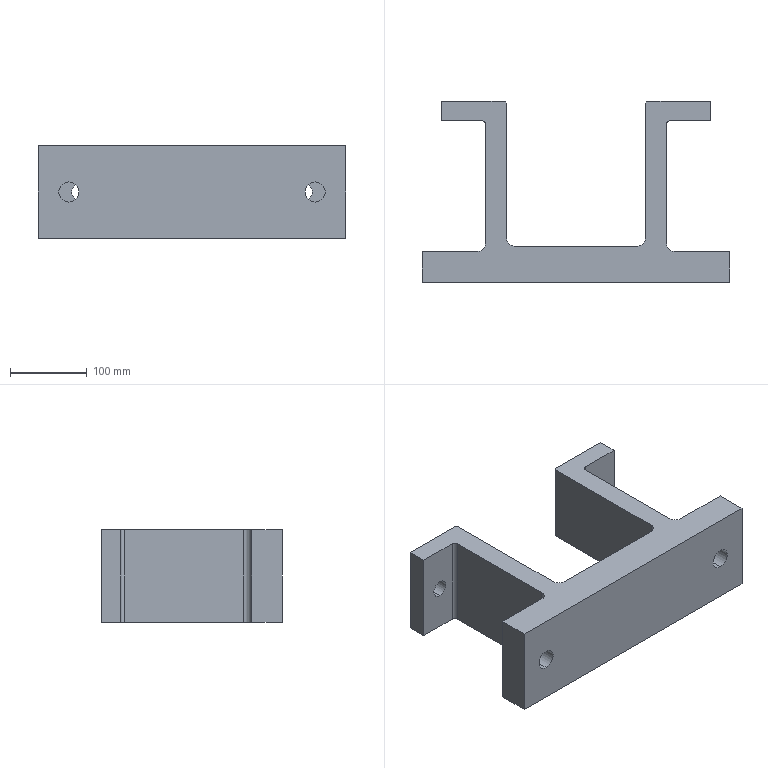Part | SolidWorks | features ICE 3, Extrusion 1 | 1 solid | 42 faces | box 400 x 235 x 120 mm | volume 3581826 mm3 | plane 25 | cylinder 17 | commonest cylinder face diameters 20 x4 22 x4 26 x4 210 x3 10 x2
STEP:
#1=CARTESIAN_POINT('',(145.,210.,-11.));
#2=VERTEX_POINT('',#1);
#3=CARTESIAN_POINT('',(145.,210.,11.));
#4=VERTEX_POINT('',#3);
#5=CARTESIAN_POINT('',(145.,210.,0.));
#6=DIRECTION('',(0.,1.,0.));
#7=DIRECTION('',(-1.,0.,0.));
#8=AXIS2_PLACEMENT_3D('',#5,#6,#7);
#9=CIRCLE('',#8,11.);
#10=EDGE_CURVE('',#2,#4,#9,.T.);
#11=ORIENTED_EDGE('',*,*,#10,.F.);
#12=CARTESIAN_POINT('',(145.,235.,-11.));
#13=VERTEX_POINT('',#12);
#14=CARTESIAN_POINT('',(145.,148.,-11.));
#15=DIRECTION('',(0.,1.,0.));
#16=VECTOR('',#15,1000.);
#17=LINE('',#14,#16);
#18=EDGE_CURVE('',#2,#13,#17,.T.);
#19=ORIENTED_EDGE('',*,*,#18,.T.);
#20=CARTESIAN_POINT('',(145.,235.,11.));
#21=VERTEX_POINT('',#20);
#22=CARTESIAN_POINT('',(145.,235.,0.));
#23=DIRECTION('',(0.,1.,0.));
#24=DIRECTION('',(0.,0.,-1.));
#25=AXIS2_PLACEMENT_3D('',#22,#23,#24);
#26=CIRCLE('',#25,11.);
#27=EDGE_CURVE('',#13,#21,#26,.T.);
#28=ORIENTED_EDGE('',*,*,#27,.T.);
#29=CARTESIAN_POINT('',(145.,148.,11.));
#30=DIRECTION('',(0.,1.,0.));
#31=VECTOR('',#30,1000.);
#32=LINE('',#29,#31);
#33=EDGE_CURVE('',#4,#21,#32,.T.);
#34=ORIENTED_EDGE('',*,*,#33,.F.);
#35=EDGE_LOOP('',(#11,#19,#28,#34));
#36=FACE_OUTER_BOUND('',#35,.T.);
#37=CARTESIAN_POINT('',(145.,148.,0.));
#38=DIRECTION('',(0.,1.,0.));
#39=DIRECTION('',(0.,0.,1.));
#40=AXIS2_PLACEMENT_3D('',#37,#38,#39);
#41=CYLINDRICAL_SURFACE('',#40,11.);
#42=ADVANCED_FACE('',(#36),#41,.F.);
#43=CARTESIAN_POINT('',(-145.,210.,-11.));
#44=VERTEX_POINT('',#43);
#45=CARTESIAN_POINT('',(-145.,210.,11.));
#46=VERTEX_POINT('',#45);
#47=CARTESIAN_POINT('',(-145.,210.,0.));
#48=DIRECTION('',(0.,1.,0.));
#49=DIRECTION('',(-1.,0.,0.));
#50=AXIS2_PLACEMENT_3D('',#47,#48,#49);
#51=CIRCLE('',#50,11.);
#52=EDGE_CURVE('',#44,#46,#51,.T.);
#53=ORIENTED_EDGE('',*,*,#52,.F.);
#54=CARTESIAN_POINT('',(-145.,235.,-11.));
#55=VERTEX_POINT('',#54);
#56=CARTESIAN_POINT('',(-145.,148.,-11.));
#57=DIRECTION('',(0.,1.,0.));
#58=VECTOR('',#57,1000.);
#59=LINE('',#56,#58);
#60=EDGE_CURVE('',#44,#55,#59,.T.);
#61=ORIENTED_EDGE('',*,*,#60,.T.);
#62=CARTESIAN_POINT('',(-145.,235.,11.));
#63=VERTEX_POINT('',#62);
#64=CARTESIAN_POINT('',(-145.,235.,0.));
#65=DIRECTION('',(0.,1.,0.));
#66=DIRECTION('',(0.,0.,1.));
#67=AXIS2_PLACEMENT_3D('',#64,#65,#66);
#68=CIRCLE('',#67,11.);
#69=EDGE_CURVE('',#55,#63,#68,.T.);
#70=ORIENTED_EDGE('',*,*,#69,.T.);
#71=CARTESIAN_POINT('',(-145.,148.,11.));
#72=DIRECTION('',(0.,1.,0.));
#73=VECTOR('',#72,1000.);
#74=LINE('',#71,#73);
#75=EDGE_CURVE('',#46,#63,#74,.T.);
#76=ORIENTED_EDGE('',*,*,#75,.F.);
#77=EDGE_LOOP('',(#53,#61,#70,#76));
#78=FACE_OUTER_BOUND('',#77,.T.);
#79=CARTESIAN_POINT('',(-145.,148.,0.));
#80=DIRECTION('',(0.,1.,0.));
#81=DIRECTION('',(0.,0.,1.));
#82=AXIS2_PLACEMENT_3D('',#79,#80,#81);
#83=CYLINDRICAL_SURFACE('',#82,11.);
#84=ADVANCED_FACE('',(#78),#83,.F.);
#85=CARTESIAN_POINT('',(-160.,40.,13.));
#86=VERTEX_POINT('',#85);
#87=CARTESIAN_POINT('',(-160.,40.,-13.));
#88=VERTEX_POINT('',#87);
#89=CARTESIAN_POINT('',(-160.,40.,0.));
#90=DIRECTION('',(0.,-1.,0.));
#91=DIRECTION('',(0.,0.,-1.));
#92=AXIS2_PLACEMENT_3D('',#89,#90,#91);
#93=CIRCLE('',#92,13.);
#94=EDGE_CURVE('',#86,#88,#93,.T.);
#95=ORIENTED_EDGE('',*,*,#94,.F.);
#96=CARTESIAN_POINT('',(-160.,0.,13.));
#97=VERTEX_POINT('',#96);
#98=CARTESIAN_POINT('',(-160.,87.,13.));
#99=DIRECTION('',(0.,-1.,0.));
#100=VECTOR('',#99,1000.);
#101=LINE('',#98,#100);
#102=EDGE_CURVE('',#86,#97,#101,.T.);
#103=ORIENTED_EDGE('',*,*,#102,.T.);
#104=CARTESIAN_POINT('',(-160.,0.,-13.));
#105=VERTEX_POINT('',#104);
#106=CARTESIAN_POINT('',(-160.,0.,0.));
#107=DIRECTION('',(0.,-1.,0.));
#108=DIRECTION('',(0.,0.,-1.));
#109=AXIS2_PLACEMENT_3D('',#106,#107,#108);
#110=CIRCLE('',#109,13.);
#111=EDGE_CURVE('',#97,#105,#110,.T.);
#112=ORIENTED_EDGE('',*,*,#111,.T.);
#113=CARTESIAN_POINT('',(-160.,87.,-13.));
#114=DIRECTION('',(0.,-1.,0.));
#115=VECTOR('',#114,1000.);
#116=LINE('',#113,#115);
#117=EDGE_CURVE('',#88,#105,#116,.T.);
#118=ORIENTED_EDGE('',*,*,#117,.F.);
#119=EDGE_LOOP('',(#95,#103,#112,#118));
#120=FACE_OUTER_BOUND('',#119,.T.);
#121=CARTESIAN_POINT('',(-160.,87.,0.));
#122=DIRECTION('',(0.,-1.,0.));
#123=DIRECTION('',(0.,0.,-1.));
#124=AXIS2_PLACEMENT_3D('',#121,#122,#123);
#125=CYLINDRICAL_SURFACE('',#124,13.);
#126=ADVANCED_FACE('',(#120),#125,.F.);
#127=CARTESIAN_POINT('',(160.,40.,13.));
#128=VERTEX_POINT('',#127);
#129=CARTESIAN_POINT('',(160.,40.,-13.));
#130=VERTEX_POINT('',#129);
#131=CARTESIAN_POINT('',(160.,40.,0.));
#132=DIRECTION('',(0.,-1.,0.));
#133=DIRECTION('',(0.,0.,-1.));
#134=AXIS2_PLACEMENT_3D('',#131,#132,#133);
#135=CIRCLE('',#134,13.);
#136=EDGE_CURVE('',#128,#130,#135,.T.);
#137=ORIENTED_EDGE('',*,*,#136,.F.);
#138=CARTESIAN_POINT('',(160.,0.,13.));
#139=VERTEX_POINT('',#138);
#140=CARTESIAN_POINT('',(160.,87.,13.));
#141=DIRECTION('',(0.,-1.,0.));
#142=VECTOR('',#141,1000.);
#143=LINE('',#140,#142);
#144=EDGE_CURVE('',#128,#139,#143,.T.);
#145=ORIENTED_EDGE('',*,*,#144,.T.);
#146=CARTESIAN_POINT('',(160.,0.,-13.));
#147=VERTEX_POINT('',#146);
#148=CARTESIAN_POINT('',(160.,0.,0.));
#149=DIRECTION('',(0.,-1.,0.));
#150=DIRECTION('',(0.,0.,1.));
#151=AXIS2_PLACEMENT_3D('',#148,#149,#150);
#152=CIRCLE('',#151,13.);
#153=EDGE_CURVE('',#139,#147,#152,.T.);
#154=ORIENTED_EDGE('',*,*,#153,.T.);
#155=CARTESIAN_POINT('',(160.,87.,-13.));
#156=DIRECTION('',(0.,-1.,0.));
#157=VECTOR('',#156,1000.);
#158=LINE('',#155,#157);
#159=EDGE_CURVE('',#130,#147,#158,.T.);
#160=ORIENTED_EDGE('',*,*,#159,.F.);
#161=EDGE_LOOP('',(#137,#145,#154,#160));
#162=FACE_OUTER_BOUND('',#161,.T.);
#163=CARTESIAN_POINT('',(160.,87.,0.));
#164=DIRECTION('',(0.,-1.,0.));
#165=DIRECTION('',(0.,0.,-1.));
#166=AXIS2_PLACEMENT_3D('',#163,#164,#165);
#167=CYLINDRICAL_SURFACE('',#166,13.);
#168=ADVANCED_FACE('',(#162),#167,.F.);
#169=CARTESIAN_POINT('',(90.,233.,-45.));
#170=VERTEX_POINT('',#169);
#171=CARTESIAN_POINT('',(92.,235.,-45.));
#172=VERTEX_POINT('',#171);
#173=CARTESIAN_POINT('',(92.,235.,-45.));
#174=DIRECTION('',(0.7071,0.7071,0.));
#175=VECTOR('',#174,1000.);
#176=LINE('',#173,#175);
#177=EDGE_CURVE('',#170,#172,#176,.T.);
#178=ORIENTED_EDGE('',*,*,#177,.F.);
#179=CARTESIAN_POINT('',(90.,233.,60.));
#180=VERTEX_POINT('',#179);
#181=CARTESIAN_POINT('',(90.,233.,60.));
#182=DIRECTION('',(0.,0.,-1.));
#183=VECTOR('',#182,1000.);
#184=LINE('',#181,#183);
#185=EDGE_CURVE('',#180,#170,#184,.T.);
#186=ORIENTED_EDGE('',*,*,#185,.F.);
#187=CARTESIAN_POINT('',(92.,235.,60.));
#188=VERTEX_POINT('',#187);
#189=CARTESIAN_POINT('',(92.,235.,60.));
#190=DIRECTION('',(-0.7071,-0.7071,0.));
#191=VECTOR('',#190,1000.);
#192=LINE('',#189,#191);
#193=EDGE_CURVE('',#188,#180,#192,.T.);
#194=ORIENTED_EDGE('',*,*,#193,.F.);
#195=CARTESIAN_POINT('',(92.,235.,60.));
#196=DIRECTION('',(0.,0.,-1.));
#197=VECTOR('',#196,1000.);
#198=LINE('',#195,#197);
#199=EDGE_CURVE('',#188,#172,#198,.T.);
#200=ORIENTED_EDGE('',*,*,#199,.T.);
#201=EDGE_LOOP('',(#178,#186,#194,#200));
#202=FACE_OUTER_BOUND('',#201,.T.);
#203=CARTESIAN_POINT('',(92.,235.,60.));
#204=DIRECTION('',(0.7071,-0.7071,0.));
#205=DIRECTION('',(0.7071,0.7071,0.));
#206=AXIS2_PLACEMENT_3D('',#203,#204,#205);
#207=PLANE('',#206);
#208=ADVANCED_FACE('',(#202),#207,.F.);
#209=CARTESIAN_POINT('',(-92.,235.,-45.));
#210=VERTEX_POINT('',#209);
#211=CARTESIAN_POINT('',(-90.,233.,-45.));
#212=VERTEX_POINT('',#211);
#213=CARTESIAN_POINT('',(-92.,235.,-45.));
#214=DIRECTION('',(0.7071,-0.7071,0.));
#215=VECTOR('',#214,1000.);
#216=LINE('',#213,#215);
#217=EDGE_CURVE('',#210,#212,#216,.T.);
#218=ORIENTED_EDGE('',*,*,#217,.F.);
#219=CARTESIAN_POINT('',(-92.,235.,60.));
#220=VERTEX_POINT('',#219);
#221=CARTESIAN_POINT('',(-92.,235.,60.));
#222=DIRECTION('',(0.,0.,-1.));
#223=VECTOR('',#222,1000.);
#224=LINE('',#221,#223);
#225=EDGE_CURVE('',#220,#210,#224,.T.);
#226=ORIENTED_EDGE('',*,*,#225,.F.);
#227=CARTESIAN_POINT('',(-90.,233.,60.));
#228=VERTEX_POINT('',#227);
#229=CARTESIAN_POINT('',(-92.,235.,60.));
#230=DIRECTION('',(-0.7071,0.7071,0.));
#231=VECTOR('',#230,1000.);
#232=LINE('',#229,#231);
#233=EDGE_CURVE('',#228,#220,#232,.T.);
#234=ORIENTED_EDGE('',*,*,#233,.F.);
#235=CARTESIAN_POINT('',(-90.,233.,60.));
#236=DIRECTION('',(0.,0.,-1.));
#237=VECTOR('',#236,1000.);
#238=LINE('',#235,#237);
#239=EDGE_CURVE('',#228,#212,#238,.T.);
#240=ORIENTED_EDGE('',*,*,#239,.T.);
#241=EDGE_LOOP('',(#218,#226,#234,#240));
#242=FACE_OUTER_BOUND('',#241,.T.);
#243=CARTESIAN_POINT('',(-92.,235.,60.));
#244=DIRECTION('',(-0.7071,-0.7071,0.));
#245=DIRECTION('',(0.7071,-0.7071,0.));
#246=AXIS2_PLACEMENT_3D('',#243,#244,#245);
#247=PLANE('',#246);
#248=ADVANCED_FACE('',(#242),#247,.F.);
#249=CARTESIAN_POINT('',(160.,40.,0.));
#250=DIRECTION('',(0.,-1.,0.));
#251=DIRECTION('',(0.,0.,-1.));
#252=AXIS2_PLACEMENT_3D('',#249,#250,#251);
#253=CIRCLE('',#252,13.);
#254=EDGE_CURVE('',#130,#128,#253,.T.);
#255=ORIENTED_EDGE('',*,*,#254,.T.);
#256=ORIENTED_EDGE('',*,*,#136,.T.);
#257=EDGE_LOOP('',(#255,#256));
#258=FACE_BOUND('',#257,.T.);
#259=CARTESIAN_POINT('',(200.,40.,-60.));
#260=VERTEX_POINT('',#259);
#261=CARTESIAN_POINT('',(127.5,40.,-60.));
#262=VERTEX_POINT('',#261);
#263=CARTESIAN_POINT('',(200.,40.,-60.));
#264=DIRECTION('',(-1.,0.,0.));
#265=VECTOR('',#264,1000.);
#266=LINE('',#263,#265);
#267=EDGE_CURVE('',#260,#262,#266,.T.);
#268=ORIENTED_EDGE('',*,*,#267,.T.);
#269=CARTESIAN_POINT('',(127.5,40.,60.));
#270=VERTEX_POINT('',#269);
#271=CARTESIAN_POINT('',(127.5,40.,60.));
#272=DIRECTION('',(0.,0.,-1.));
#273=VECTOR('',#272,1000.);
#274=LINE('',#271,#273);
#275=EDGE_CURVE('',#270,#262,#274,.T.);
#276=ORIENTED_EDGE('',*,*,#275,.F.);
#277=CARTESIAN_POINT('',(200.,40.,60.));
#278=VERTEX_POINT('',#277);
#279=CARTESIAN_POINT('',(200.,40.,60.));
#280=DIRECTION('',(-1.,0.,0.));
#281=VECTOR('',#280,1000.);
#282=LINE('',#279,#281);
#283=EDGE_CURVE('',#278,#270,#282,.T.);
#284=ORIENTED_EDGE('',*,*,#283,.F.);
#285=CARTESIAN_POINT('',(200.,40.,60.));
#286=DIRECTION('',(0.,0.,-1.));
#287=VECTOR('',#286,1000.);
#288=LINE('',#285,#287);
#289=EDGE_CURVE('',#278,#260,#288,.T.);
#290=ORIENTED_EDGE('',*,*,#289,.T.);
#291=EDGE_LOOP('',(#268,#276,#284,#290));
#292=FACE_OUTER_BOUND('',#291,.T.);
#293=CARTESIAN_POINT('',(200.,40.,60.));
#294=DIRECTION('',(0.,-1.,0.));
#295=DIRECTION('',(0.,0.,-1.));
#296=AXIS2_PLACEMENT_3D('',#293,#294,#295);
#297=PLANE('',#296);
#298=ADVANCED_FACE('',(#258,#292),#297,.F.);
#299=CARTESIAN_POINT('',(117.5,50.,-60.));
#300=VERTEX_POINT('',#299);
#301=CARTESIAN_POINT('',(127.5,50.,-60.));
#302=DIRECTION('',(0.,0.,-1.));
#303=DIRECTION('',(-1.,0.,0.));
#304=AXIS2_PLACEMENT_3D('',#301,#302,#303);
#305=CIRCLE('',#304,10.);
#306=EDGE_CURVE('',#262,#300,#305,.T.);
#307=ORIENTED_EDGE('',*,*,#306,.T.);
#308=CARTESIAN_POINT('',(117.5,50.,60.));
#309=VERTEX_POINT('',#308);
#310=CARTESIAN_POINT('',(117.5,50.,60.));
#311=DIRECTION('',(0.,0.,-1.));
#312=VECTOR('',#311,1000.);
#313=LINE('',#310,#312);
#314=EDGE_CURVE('',#309,#300,#313,.T.);
#315=ORIENTED_EDGE('',*,*,#314,.F.);
#316=CARTESIAN_POINT('',(127.5,50.,60.));
#317=DIRECTION('',(0.,0.,-1.));
#318=DIRECTION('',(-1.,0.,0.));
#319=AXIS2_PLACEMENT_3D('',#316,#317,#318);
#320=CIRCLE('',#319,10.);
#321=EDGE_CURVE('',#270,#309,#320,.T.);
#322=ORIENTED_EDGE('',*,*,#321,.F.);
#323=ORIENTED_EDGE('',*,*,#275,.T.);
#324=EDGE_LOOP('',(#307,#315,#322,#323));
#325=FACE_OUTER_BOUND('',#324,.T.);
#326=CARTESIAN_POINT('',(127.5,50.,60.));
#327=DIRECTION('',(0.,0.,-1.));
#328=DIRECTION('',(-1.,0.,0.));
#329=AXIS2_PLACEMENT_3D('',#326,#327,#328);
#330=CYLINDRICAL_SURFACE('',#329,10.);
#331=ADVANCED_FACE('',(#325),#330,.F.);
#332=CARTESIAN_POINT('',(117.5,205.,-60.));
#333=VERTEX_POINT('',#332);
#334=CARTESIAN_POINT('',(117.5,50.,-60.));
#335=DIRECTION('',(0.,1.,0.));
#336=VECTOR('',#335,1000.);
#337=LINE('',#334,#336);
#338=EDGE_CURVE('',#300,#333,#337,.T.);
#339=ORIENTED_EDGE('',*,*,#338,.T.);
#340=CARTESIAN_POINT('',(117.5,205.,60.));
#341=VERTEX_POINT('',#340);
#342=CARTESIAN_POINT('',(117.5,205.,60.));
#343=DIRECTION('',(0.,0.,-1.));
#344=VECTOR('',#343,1000.);
#345=LINE('',#342,#344);
#346=EDGE_CURVE('',#341,#333,#345,.T.);
#347=ORIENTED_EDGE('',*,*,#346,.F.);
#348=CARTESIAN_POINT('',(117.5,50.,60.));
#349=DIRECTION('',(0.,1.,0.));
#350=VECTOR('',#349,1000.);
#351=LINE('',#348,#350);
#352=EDGE_CURVE('',#309,#341,#351,.T.);
#353=ORIENTED_EDGE('',*,*,#352,.F.);
#354=ORIENTED_EDGE('',*,*,#314,.T.);
#355=EDGE_LOOP('',(#339,#347,#353,#354));
#356=FACE_OUTER_BOUND('',#355,.T.);
#357=CARTESIAN_POINT('',(117.5,50.,60.));
#358=DIRECTION('',(-1.,0.,0.));
#359=DIRECTION('',(0.,0.,1.));
#360=AXIS2_PLACEMENT_3D('',#357,#358,#359);
#361=PLANE('',#360);
#362=ADVANCED_FACE('',(#356),#361,.F.);
#363=CARTESIAN_POINT('',(122.5,210.,-60.));
#364=VERTEX_POINT('',#363);
#365=CARTESIAN_POINT('',(122.5,205.,-60.));
#366=DIRECTION('',(0.,0.,-1.));
#367=DIRECTION('',(1.,0.,0.));
#368=AXIS2_PLACEMENT_3D('',#365,#366,#367);
#369=CIRCLE('',#368,5.);
#370=EDGE_CURVE('',#333,#364,#369,.T.);
#371=ORIENTED_EDGE('',*,*,#370,.T.);
#372=CARTESIAN_POINT('',(122.5,210.,60.));
#373=VERTEX_POINT('',#372);
#374=CARTESIAN_POINT('',(122.5,210.,60.));
#375=DIRECTION('',(0.,0.,-1.));
#376=VECTOR('',#375,1000.);
#377=LINE('',#374,#376);
#378=EDGE_CURVE('',#373,#364,#377,.T.);
#379=ORIENTED_EDGE('',*,*,#378,.F.);
#380=CARTESIAN_POINT('',(122.5,205.,60.));
#381=DIRECTION('',(0.,0.,-1.));
#382=DIRECTION('',(1.,0.,0.));
#383=AXIS2_PLACEMENT_3D('',#380,#381,#382);
#384=CIRCLE('',#383,5.);
#385=EDGE_CURVE('',#341,#373,#384,.T.);
#386=ORIENTED_EDGE('',*,*,#385,.F.);
#387=ORIENTED_EDGE('',*,*,#346,.T.);
#388=EDGE_LOOP('',(#371,#379,#386,#387));
#389=FACE_OUTER_BOUND('',#388,.T.);
#390=CARTESIAN_POINT('',(122.5,205.,60.));
#391=DIRECTION('',(0.,0.,-1.));
#392=DIRECTION('',(-1.,0.,0.));
#393=AXIS2_PLACEMENT_3D('',#390,#391,#392);
#394=CYLINDRICAL_SURFACE('',#393,5.);
#395=ADVANCED_FACE('',(#389),#394,.F.);
#396=CARTESIAN_POINT('',(145.,210.,0.));
#397=DIRECTION('',(0.,1.,0.));
#398=DIRECTION('',(-1.,0.,0.));
#399=AXIS2_PLACEMENT_3D('',#396,#397,#398);
#400=CIRCLE('',#399,11.);
#401=EDGE_CURVE('',#4,#2,#400,.T.);
#402=ORIENTED_EDGE('',*,*,#401,.T.);
#403=ORIENTED_EDGE('',*,*,#10,.T.);
#404=EDGE_LOOP('',(#402,#403));
#405=FACE_BOUND('',#404,.T.);
#406=CARTESIAN_POINT('',(175.,210.,-60.));
#407=VERTEX_POINT('',#406);
#408=CARTESIAN_POINT('',(122.5,210.,-60.));
#409=DIRECTION('',(1.,0.,0.));
#410=VECTOR('',#409,1000.);
#411=LINE('',#408,#410);
#412=EDGE_CURVE('',#364,#407,#411,.T.);
#413=ORIENTED_EDGE('',*,*,#412,.T.);
#414=CARTESIAN_POINT('',(175.,210.,60.));
#415=VERTEX_POINT('',#414);
#416=CARTESIAN_POINT('',(175.,210.,60.));
#417=DIRECTION('',(0.,0.,-1.));
#418=VECTOR('',#417,1000.);
#419=LINE('',#416,#418);
#420=EDGE_CURVE('',#415,#407,#419,.T.);
#421=ORIENTED_EDGE('',*,*,#420,.F.);
#422=CARTESIAN_POINT('',(122.5,210.,60.));
#423=DIRECTION('',(1.,0.,0.));
#424=VECTOR('',#423,1000.);
#425=LINE('',#422,#424);
#426=EDGE_CURVE('',#373,#415,#425,.T.);
#427=ORIENTED_EDGE('',*,*,#426,.F.);
#428=ORIENTED_EDGE('',*,*,#378,.T.);
#429=EDGE_LOOP('',(#413,#421,#427,#428));
#430=FACE_OUTER_BOUND('',#429,.T.);
#431=CARTESIAN_POINT('',(122.5,210.,60.));
#432=DIRECTION('',(0.,1.,0.));
#433=DIRECTION('',(-1.,0.,0.));
#434=AXIS2_PLACEMENT_3D('',#431,#432,#433);
#435=PLANE('',#434);
#436=ADVANCED_FACE('',(#405,#430),#435,.F.);
#437=CARTESIAN_POINT('',(175.,235.,-60.));
#438=VERTEX_POINT('',#437);
#439=CARTESIAN_POINT('',(175.,210.,-60.));
#440=DIRECTION('',(0.,1.,0.));
#441=VECTOR('',#440,1000.);
#442=LINE('',#439,#441);
#443=EDGE_CURVE('',#407,#438,#442,.T.);
#444=ORIENTED_EDGE('',*,*,#443,.T.);
#445=CARTESIAN_POINT('',(175.,235.,60.));
#446=VERTEX_POINT('',#445);
#447=CARTESIAN_POINT('',(175.,235.,60.));
#448=DIRECTION('',(0.,0.,-1.));
#449=VECTOR('',#448,1000.);
#450=LINE('',#447,#449);
#451=EDGE_CURVE('',#446,#438,#450,.T.);
#452=ORIENTED_EDGE('',*,*,#451,.F.);
#453=CARTESIAN_POINT('',(175.,210.,60.));
#454=DIRECTION('',(0.,1.,0.));
#455=VECTOR('',#454,1000.);
#456=LINE('',#453,#455);
#457=EDGE_CURVE('',#415,#446,#456,.T.);
#458=ORIENTED_EDGE('',*,*,#457,.F.);
#459=ORIENTED_EDGE('',*,*,#420,.T.);
#460=EDGE_LOOP('',(#444,#452,#458,#459));
#461=FACE_OUTER_BOUND('',#460,.T.);
#462=CARTESIAN_POINT('',(175.,210.,60.));
#463=DIRECTION('',(-1.,0.,0.));
#464=DIRECTION('',(0.,0.,1.));
#465=AXIS2_PLACEMENT_3D('',#462,#463,#464);
#466=PLANE('',#465);
#467=ADVANCED_FACE('',(#461),#466,.F.);
#468=CARTESIAN_POINT('',(145.,235.,0.));
#469=DIRECTION('',(0.,1.,0.));
#470=DIRECTION('',(0.,0.,-1.));
#471=AXIS2_PLACEMENT_3D('',#468,#469,#470);
#472=CIRCLE('',#471,11.);
#473=EDGE_CURVE('',#21,#13,#472,.T.);
#474=ORIENTED_EDGE('',*,*,#473,.F.);
#475=ORIENTED_EDGE('',*,*,#27,.F.);
#476=EDGE_LOOP('',(#474,#475));
#477=FACE_BOUND('',#476,.T.);
#478=CARTESIAN_POINT('',(105.,235.,-60.));
#479=VERTEX_POINT('',#478);
#480=CARTESIAN_POINT('',(175.,235.,-60.));
#481=DIRECTION('',(-1.,0.,0.));
#482=VECTOR('',#481,1000.);
#483=LINE('',#480,#482);
#484=EDGE_CURVE('',#438,#479,#483,.T.);
#485=ORIENTED_EDGE('',*,*,#484,.T.);
#486=CARTESIAN_POINT('',(105.,235.,-45.));
#487=VERTEX_POINT('',#486);
#488=CARTESIAN_POINT('',(105.,235.,60.));
#489=DIRECTION('',(0.,0.,1.));
#490=VECTOR('',#489,1000.);
#491=LINE('',#488,#490);
#492=EDGE_CURVE('',#479,#487,#491,.T.);
#493=ORIENTED_EDGE('',*,*,#492,.T.);
#494=CARTESIAN_POINT('',(175.,235.,-45.));
#495=DIRECTION('',(1.,0.,0.));
#496=VECTOR('',#495,1000.);
#497=LINE('',#494,#496);
#498=EDGE_CURVE('',#172,#487,#497,.T.);
#499=ORIENTED_EDGE('',*,*,#498,.F.);
#500=ORIENTED_EDGE('',*,*,#199,.F.);
#501=CARTESIAN_POINT('',(175.,235.,60.));
#502=DIRECTION('',(-1.,0.,0.));
#503=VECTOR('',#502,1000.);
#504=LINE('',#501,#503);
#505=EDGE_CURVE('',#446,#188,#504,.T.);
#506=ORIENTED_EDGE('',*,*,#505,.F.);
#507=ORIENTED_EDGE('',*,*,#451,.T.);
#508=EDGE_LOOP('',(#485,#493,#499,#500,#506,#507));
#509=FACE_OUTER_BOUND('',#508,.T.);
#510=CARTESIAN_POINT('',(175.,235.,60.));
#511=DIRECTION('',(0.,-1.,0.));
#512=DIRECTION('',(0.,0.,-1.));
#513=AXIS2_PLACEMENT_3D('',#510,#511,#512);
#514=PLANE('',#513);
#515=ADVANCED_FACE('',(#477,#509),#514,.F.);
#516=CARTESIAN_POINT('',(90.,85.917,-45.));
#517=VERTEX_POINT('',#516);
#518=CARTESIAN_POINT('',(90.,233.,-45.));
#519=DIRECTION('',(0.,1.,0.));
#520=VECTOR('',#519,1000.);
#521=LINE('',#518,#520);
#522=EDGE_CURVE('',#517,#170,#521,.T.);
#523=ORIENTED_EDGE('',*,*,#522,.F.);
#524=CARTESIAN_POINT('',(90.,85.917,-60.));
#525=VERTEX_POINT('',#524);
#526=CARTESIAN_POINT('',(90.,85.917,-45.));
#527=DIRECTION('',(0.,0.,-1.));
#528=VECTOR('',#527,1000.);
#529=LINE('',#526,#528);
#530=EDGE_CURVE('',#517,#525,#529,.T.);
#531=ORIENTED_EDGE('',*,*,#530,.T.);
#532=CARTESIAN_POINT('',(90.,57.,-60.));
#533=VERTEX_POINT('',#532);
#534=CARTESIAN_POINT('',(90.,233.,-60.));
#535=DIRECTION('',(0.,-1.,0.));
#536=VECTOR('',#535,1000.);
#537=LINE('',#534,#536);
#538=EDGE_CURVE('',#525,#533,#537,.T.);
#539=ORIENTED_EDGE('',*,*,#538,.T.);
#540=CARTESIAN_POINT('',(90.,57.,60.));
#541=VERTEX_POINT('',#540);
#542=CARTESIAN_POINT('',(90.,57.,60.));
#543=DIRECTION('',(0.,0.,-1.));
#544=VECTOR('',#543,1000.);
#545=LINE('',#542,#544);
#546=EDGE_CURVE('',#541,#533,#545,.T.);
#547=ORIENTED_EDGE('',*,*,#546,.F.);
#548=CARTESIAN_POINT('',(90.,233.,60.));
#549=DIRECTION('',(0.,-1.,0.));
#550=VECTOR('',#549,1000.);
#551=LINE('',#548,#550);
#552=EDGE_CURVE('',#180,#541,#551,.T.);
#553=ORIENTED_EDGE('',*,*,#552,.F.);
#554=ORIENTED_EDGE('',*,*,#185,.T.);
#555=EDGE_LOOP('',(#523,#531,#539,#547,#553,#554));
#556=FACE_OUTER_BOUND('',#555,.T.);
#557=CARTESIAN_POINT('',(90.,233.,60.));
#558=DIRECTION('',(1.,0.,0.));
#559=DIRECTION('',(0.,1.,0.));
#560=AXIS2_PLACEMENT_3D('',#557,#558,#559);
#561=PLANE('',#560);
#562=ADVANCED_FACE('',(#556),#561,.F.);
#563=CARTESIAN_POINT('',(80.,47.,-60.));
#564=VERTEX_POINT('',#563);
#565=CARTESIAN_POINT('',(80.,57.,-60.));
#566=DIRECTION('',(0.,0.,-1.));
#567=DIRECTION('',(1.,0.,0.));
#568=AXIS2_PLACEMENT_3D('',#565,#566,#567);
#569=CIRCLE('',#568,10.);
#570=EDGE_CURVE('',#533,#564,#569,.T.);
#571=ORIENTED_EDGE('',*,*,#570,.T.);
#572=CARTESIAN_POINT('',(80.,47.,60.));
#573=VERTEX_POINT('',#572);
#574=CARTESIAN_POINT('',(80.,47.,60.));
#575=DIRECTION('',(0.,0.,-1.));
#576=VECTOR('',#575,1000.);
#577=LINE('',#574,#576);
#578=EDGE_CURVE('',#573,#564,#577,.T.);
#579=ORIENTED_EDGE('',*,*,#578,.F.);
#580=CARTESIAN_POINT('',(80.,57.,60.));
#581=DIRECTION('',(0.,0.,-1.));
#582=DIRECTION('',(1.,0.,0.));
#583=AXIS2_PLACEMENT_3D('',#580,#581,#582);
#584=CIRCLE('',#583,10.);
#585=EDGE_CURVE('',#541,#573,#584,.T.);
#586=ORIENTED_EDGE('',*,*,#585,.F.);
#587=ORIENTED_EDGE('',*,*,#546,.T.);
#588=EDGE_LOOP('',(#571,#579,#586,#587));
#589=FACE_OUTER_BOUND('',#588,.T.);
#590=CARTESIAN_POINT('',(80.,57.,60.));
#591=DIRECTION('',(0.,0.,-1.));
#592=DIRECTION('',(-1.,0.,0.));
#593=AXIS2_PLACEMENT_3D('',#590,#591,#592);
#594=CYLINDRICAL_SURFACE('',#593,10.);
#595=ADVANCED_FACE('',(#589),#594,.F.);
#596=CARTESIAN_POINT('',(-48.744,47.,-45.));
#597=VERTEX_POINT('',#596);
#598=CARTESIAN_POINT('',(48.744,47.,-45.));
#599=VERTEX_POINT('',#598);
#600=CARTESIAN_POINT('',(-80.,47.,-45.));
#601=DIRECTION('',(1.,0.,0.));
#602=VECTOR('',#601,1000.);
#603=LINE('',#600,#602);
#604=EDGE_CURVE('',#597,#599,#603,.T.);
#605=ORIENTED_EDGE('',*,*,#604,.F.);
#606=CARTESIAN_POINT('',(-48.744,47.,-60.));
#607=VERTEX_POINT('',#606);
#608=CARTESIAN_POINT('',(-48.744,47.,-45.));
#609=DIRECTION('',(0.,0.,-1.));
#610=VECTOR('',#609,1000.);
#611=LINE('',#608,#610);
#612=EDGE_CURVE('',#597,#607,#611,.T.);
#613=ORIENTED_EDGE('',*,*,#612,.T.);
#614=CARTESIAN_POINT('',(-80.,47.,-60.));
#615=VERTEX_POINT('',#614);
#616=CARTESIAN_POINT('',(-80.,47.,-60.));
#617=DIRECTION('',(-1.,0.,0.));
#618=VECTOR('',#617,1000.);
#619=LINE('',#616,#618);
#620=EDGE_CURVE('',#607,#615,#619,.T.);
#621=ORIENTED_EDGE('',*,*,#620,.T.);
#622=CARTESIAN_POINT('',(-80.,47.,60.));
#623=VERTEX_POINT('',#622);
#624=CARTESIAN_POINT('',(-80.,47.,60.));
#625=DIRECTION('',(0.,0.,-1.));
#626=VECTOR('',#625,1000.);
#627=LINE('',#624,#626);
#628=EDGE_CURVE('',#623,#615,#627,.T.);
#629=ORIENTED_EDGE('',*,*,#628,.F.);
#630=CARTESIAN_POINT('',(-80.,47.,60.));
#631=DIRECTION('',(-1.,0.,0.));
#632=VECTOR('',#631,1000.);
#633=LINE('',#630,#632);
#634=EDGE_CURVE('',#573,#623,#633,.T.);
#635=ORIENTED_EDGE('',*,*,#634,.F.);
#636=ORIENTED_EDGE('',*,*,#578,.T.);
#637=CARTESIAN_POINT('',(48.744,47.,-60.));
#638=VERTEX_POINT('',#637);
#639=CARTESIAN_POINT('',(-80.,47.,-60.));
#640=DIRECTION('',(-1.,0.,0.));
#641=VECTOR('',#640,1000.);
#642=LINE('',#639,#641);
#643=EDGE_CURVE('',#564,#638,#642,.T.);
#644=ORIENTED_EDGE('',*,*,#643,.T.);
#645=CARTESIAN_POINT('',(48.744,47.,-45.));
#646=DIRECTION('',(0.,0.,1.));
#647=VECTOR('',#646,1000.);
#648=LINE('',#645,#647);
#649=EDGE_CURVE('',#638,#599,#648,.T.);
#650=ORIENTED_EDGE('',*,*,#649,.T.);
#651=EDGE_LOOP('',(#605,#613,#621,#629,#635,#636,#644,#650));
#652=FACE_OUTER_BOUND('',#651,.T.);
#653=CARTESIAN_POINT('',(-80.,47.,60.));
#654=DIRECTION('',(0.,-1.,0.));
#655=DIRECTION('',(0.,0.,-1.));
#656=AXIS2_PLACEMENT_3D('',#653,#654,#655);
#657=PLANE('',#656);
#658=ADVANCED_FACE('',(#652),#657,.F.);
#659=CARTESIAN_POINT('',(-90.,57.,-60.));
#660=VERTEX_POINT('',#659);
#661=CARTESIAN_POINT('',(-80.,57.,-60.));
#662=DIRECTION('',(0.,0.,-1.));
#663=DIRECTION('',(-1.,0.,0.));
#664=AXIS2_PLACEMENT_3D('',#661,#662,#663);
#665=CIRCLE('',#664,10.);
#666=EDGE_CURVE('',#615,#660,#665,.T.);
#667=ORIENTED_EDGE('',*,*,#666,.T.);
#668=CARTESIAN_POINT('',(-90.,57.,60.));
#669=VERTEX_POINT('',#668);
#670=CARTESIAN_POINT('',(-90.,57.,60.));
#671=DIRECTION('',(0.,0.,-1.));
#672=VECTOR('',#671,1000.);
#673=LINE('',#670,#672);
#674=EDGE_CURVE('',#669,#660,#673,.T.);
#675=ORIENTED_EDGE('',*,*,#674,.F.);
#676=CARTESIAN_POINT('',(-80.,57.,60.));
#677=DIRECTION('',(0.,0.,-1.));
#678=DIRECTION('',(-1.,0.,0.));
#679=AXIS2_PLACEMENT_3D('',#676,#677,#678);
#680=CIRCLE('',#679,10.);
#681=EDGE_CURVE('',#623,#669,#680,.T.);
#682=ORIENTED_EDGE('',*,*,#681,.F.);
#683=ORIENTED_EDGE('',*,*,#628,.T.);
#684=EDGE_LOOP('',(#667,#675,#682,#683));
#685=FACE_OUTER_BOUND('',#684,.T.);
#686=CARTESIAN_POINT('',(-80.,57.,60.));
#687=DIRECTION('',(0.,0.,-1.));
#688=DIRECTION('',(-1.,0.,0.));
#689=AXIS2_PLACEMENT_3D('',#686,#687,#688);
#690=CYLINDRICAL_SURFACE('',#689,10.);
#691=ADVANCED_FACE('',(#685),#690,.F.);
#692=CARTESIAN_POINT('',(-90.,85.917,-60.));
#693=VERTEX_POINT('',#692);
#694=CARTESIAN_POINT('',(-90.,233.,-60.));
#695=DIRECTION('',(0.,1.,0.));
#696=VECTOR('',#695,1000.);
#697=LINE('',#694,#696);
#698=EDGE_CURVE('',#660,#693,#697,.T.);
#699=ORIENTED_EDGE('',*,*,#698,.T.);
#700=CARTESIAN_POINT('',(-90.,85.917,-45.));
#701=VERTEX_POINT('',#700);
#702=CARTESIAN_POINT('',(-90.,85.917,-45.));
#703=DIRECTION('',(0.,0.,1.));
#704=VECTOR('',#703,1000.);
#705=LINE('',#702,#704);
#706=EDGE_CURVE('',#693,#701,#705,.T.);
#707=ORIENTED_EDGE('',*,*,#706,.T.);
#708=CARTESIAN_POINT('',(-90.,233.,-45.));
#709=DIRECTION('',(0.,-1.,0.));
#710=VECTOR('',#709,1000.);
#711=LINE('',#708,#710);
#712=EDGE_CURVE('',#212,#701,#711,.T.);
#713=ORIENTED_EDGE('',*,*,#712,.F.);
#714=ORIENTED_EDGE('',*,*,#239,.F.);
#715=CARTESIAN_POINT('',(-90.,233.,60.));
#716=DIRECTION('',(0.,1.,0.));
#717=VECTOR('',#716,1000.);
#718=LINE('',#715,#717);
#719=EDGE_CURVE('',#669,#228,#718,.T.);
#720=ORIENTED_EDGE('',*,*,#719,.F.);
#721=ORIENTED_EDGE('',*,*,#674,.T.);
#722=EDGE_LOOP('',(#699,#707,#713,#714,#720,#721));
#723=FACE_OUTER_BOUND('',#722,.T.);
#724=CARTESIAN_POINT('',(-90.,233.,60.));
#725=DIRECTION('',(-1.,0.,0.));
#726=DIRECTION('',(0.,-1.,0.));
#727=AXIS2_PLACEMENT_3D('',#724,#725,#726);
#728=PLANE('',#727);
#729=ADVANCED_FACE('',(#723),#728,.F.);
#730=CARTESIAN_POINT('',(-145.,235.,0.));
#731=DIRECTION('',(0.,1.,0.));
#732=DIRECTION('',(0.,0.,1.));
#733=AXIS2_PLACEMENT_3D('',#730,#731,#732);
#734=CIRCLE('',#733,11.);
#735=EDGE_CURVE('',#63,#55,#734,.T.);
#736=ORIENTED_EDGE('',*,*,#735,.F.);
#737=ORIENTED_EDGE('',*,*,#69,.F.);
#738=EDGE_LOOP('',(#736,#737));
#739=FACE_BOUND('',#738,.T.);
#740=CARTESIAN_POINT('',(-105.,235.,-45.));
#741=VERTEX_POINT('',#740);
#742=CARTESIAN_POINT('',(-175.,235.,-45.));
#743=DIRECTION('',(1.,0.,0.));
#744=VECTOR('',#743,1000.);
#745=LINE('',#742,#744);
#746=EDGE_CURVE('',#741,#210,#745,.T.);
#747=ORIENTED_EDGE('',*,*,#746,.F.);
#748=CARTESIAN_POINT('',(-105.,235.,-60.));
#749=VERTEX_POINT('',#748);
#750=CARTESIAN_POINT('',(-105.,235.,60.));
#751=DIRECTION('',(0.,0.,-1.));
#752=VECTOR('',#751,1000.);
#753=LINE('',#750,#752);
#754=EDGE_CURVE('',#741,#749,#753,.T.);
#755=ORIENTED_EDGE('',*,*,#754,.T.);
#756=CARTESIAN_POINT('',(-175.,235.,-60.));
#757=VERTEX_POINT('',#756);
#758=CARTESIAN_POINT('',(-175.,235.,-60.));
#759=DIRECTION('',(-1.,0.,0.));
#760=VECTOR('',#759,1000.);
#761=LINE('',#758,#760);
#762=EDGE_CURVE('',#749,#757,#761,.T.);
#763=ORIENTED_EDGE('',*,*,#762,.T.);
#764=CARTESIAN_POINT('',(-175.,235.,60.));
#765=VERTEX_POINT('',#764);
#766=CARTESIAN_POINT('',(-175.,235.,60.));
#767=DIRECTION('',(0.,0.,-1.));
#768=VECTOR('',#767,1000.);
#769=LINE('',#766,#768);
#770=EDGE_CURVE('',#765,#757,#769,.T.);
#771=ORIENTED_EDGE('',*,*,#770,.F.);
#772=CARTESIAN_POINT('',(-175.,235.,60.));
#773=DIRECTION('',(-1.,0.,0.));
#774=VECTOR('',#773,1000.);
#775=LINE('',#772,#774);
#776=EDGE_CURVE('',#220,#765,#775,.T.);
#777=ORIENTED_EDGE('',*,*,#776,.F.);
#778=ORIENTED_EDGE('',*,*,#225,.T.);
#779=EDGE_LOOP('',(#747,#755,#763,#771,#777,#778));
#780=FACE_OUTER_BOUND('',#779,.T.);
#781=CARTESIAN_POINT('',(-175.,235.,60.));
#782=DIRECTION('',(0.,-1.,0.));
#783=DIRECTION('',(0.,0.,-1.));
#784=AXIS2_PLACEMENT_3D('',#781,#782,#783);
#785=PLANE('',#784);
#786=ADVANCED_FACE('',(#739,#780),#785,.F.);
#787=CARTESIAN_POINT('',(-175.,210.,-60.));
#788=VERTEX_POINT('',#787);
#789=CARTESIAN_POINT('',(-175.,210.,-60.));
#790=DIRECTION('',(0.,-1.,0.));
#791=VECTOR('',#790,1000.);
#792=LINE('',#789,#791);
#793=EDGE_CURVE('',#757,#788,#792,.T.);
#794=ORIENTED_EDGE('',*,*,#793,.T.);
#795=CARTESIAN_POINT('',(-175.,210.,60.));
#796=VERTEX_POINT('',#795);
#797=CARTESIAN_POINT('',(-175.,210.,60.));
#798=DIRECTION('',(0.,0.,-1.));
#799=VECTOR('',#798,1000.);
#800=LINE('',#797,#799);
#801=EDGE_CURVE('',#796,#788,#800,.T.);
#802=ORIENTED_EDGE('',*,*,#801,.F.);
#803=CARTESIAN_POINT('',(-175.,210.,60.));
#804=DIRECTION('',(0.,-1.,0.));
#805=VECTOR('',#804,1000.);
#806=LINE('',#803,#805);
#807=EDGE_CURVE('',#765,#796,#806,.T.);
#808=ORIENTED_EDGE('',*,*,#807,.F.);
#809=ORIENTED_EDGE('',*,*,#770,.T.);
#810=EDGE_LOOP('',(#794,#802,#808,#809));
#811=FACE_OUTER_BOUND('',#810,.T.);
#812=CARTESIAN_POINT('',(-175.,210.,60.));
#813=DIRECTION('',(1.,0.,0.));
#814=DIRECTION('',(0.,0.,-1.));
#815=AXIS2_PLACEMENT_3D('',#812,#813,#814);
#816=PLANE('',#815);
#817=ADVANCED_FACE('',(#811),#816,.F.);
#818=CARTESIAN_POINT('',(-145.,210.,0.));
#819=DIRECTION('',(0.,1.,0.));
#820=DIRECTION('',(-1.,0.,0.));
#821=AXIS2_PLACEMENT_3D('',#818,#819,#820);
#822=CIRCLE('',#821,11.);
#823=EDGE_CURVE('',#46,#44,#822,.T.);
#824=ORIENTED_EDGE('',*,*,#823,.T.);
#825=ORIENTED_EDGE('',*,*,#52,.T.);
#826=EDGE_LOOP('',(#824,#825));
#827=FACE_BOUND('',#826,.T.);
#828=CARTESIAN_POINT('',(-122.5,210.,-60.));
#829=VERTEX_POINT('',#828);
#830=CARTESIAN_POINT('',(-122.5,210.,-60.));
#831=DIRECTION('',(1.,0.,0.));
#832=VECTOR('',#831,1000.);
#833=LINE('',#830,#832);
#834=EDGE_CURVE('',#788,#829,#833,.T.);
#835=ORIENTED_EDGE('',*,*,#834,.T.);
#836=CARTESIAN_POINT('',(-122.5,210.,60.));
#837=VERTEX_POINT('',#836);
#838=CARTESIAN_POINT('',(-122.5,210.,60.));
#839=DIRECTION('',(0.,0.,-1.));
#840=VECTOR('',#839,1000.);
#841=LINE('',#838,#840);
#842=EDGE_CURVE('',#837,#829,#841,.T.);
#843=ORIENTED_EDGE('',*,*,#842,.F.);
#844=CARTESIAN_POINT('',(-122.5,210.,60.));
#845=DIRECTION('',(1.,0.,0.));
#846=VECTOR('',#845,1000.);
#847=LINE('',#844,#846);
#848=EDGE_CURVE('',#796,#837,#847,.T.);
#849=ORIENTED_EDGE('',*,*,#848,.F.);
#850=ORIENTED_EDGE('',*,*,#801,.T.);
#851=EDGE_LOOP('',(#835,#843,#849,#850));
#852=FACE_OUTER_BOUND('',#851,.T.);
#853=CARTESIAN_POINT('',(-122.5,210.,60.));
#854=DIRECTION('',(0.,1.,0.));
#855=DIRECTION('',(-1.,0.,0.));
#856=AXIS2_PLACEMENT_3D('',#853,#854,#855);
#857=PLANE('',#856);
#858=ADVANCED_FACE('',(#827,#852),#857,.F.);
#859=CARTESIAN_POINT('',(-117.5,205.,-60.));
#860=VERTEX_POINT('',#859);
#861=CARTESIAN_POINT('',(-122.5,205.,-60.));
#862=DIRECTION('',(0.,0.,-1.));
#863=DIRECTION('',(1.,0.,0.));
#864=AXIS2_PLACEMENT_3D('',#861,#862,#863);
#865=CIRCLE('',#864,5.);
#866=EDGE_CURVE('',#829,#860,#865,.T.);
#867=ORIENTED_EDGE('',*,*,#866,.T.);
#868=CARTESIAN_POINT('',(-117.5,205.,60.));
#869=VERTEX_POINT('',#868);
#870=CARTESIAN_POINT('',(-117.5,205.,60.));
#871=DIRECTION('',(0.,0.,-1.));
#872=VECTOR('',#871,1000.);
#873=LINE('',#870,#872);
#874=EDGE_CURVE('',#869,#860,#873,.T.);
#875=ORIENTED_EDGE('',*,*,#874,.F.);
#876=CARTESIAN_POINT('',(-122.5,205.,60.));
#877=DIRECTION('',(0.,0.,-1.));
#878=DIRECTION('',(1.,0.,0.));
#879=AXIS2_PLACEMENT_3D('',#876,#877,#878);
#880=CIRCLE('',#879,5.);
#881=EDGE_CURVE('',#837,#869,#880,.T.);
#882=ORIENTED_EDGE('',*,*,#881,.F.);
#883=ORIENTED_EDGE('',*,*,#842,.T.);
#884=EDGE_LOOP('',(#867,#875,#882,#883));
#885=FACE_OUTER_BOUND('',#884,.T.);
#886=CARTESIAN_POINT('',(-122.5,205.,60.));
#887=DIRECTION('',(0.,0.,-1.));
#888=DIRECTION('',(-1.,0.,0.));
#889=AXIS2_PLACEMENT_3D('',#886,#887,#888);
#890=CYLINDRICAL_SURFACE('',#889,5.);
#891=ADVANCED_FACE('',(#885),#890,.F.);
#892=CARTESIAN_POINT('',(-117.5,50.,-60.));
#893=VERTEX_POINT('',#892);
#894=CARTESIAN_POINT('',(-117.5,50.,-60.));
#895=DIRECTION('',(0.,-1.,0.));
#896=VECTOR('',#895,1000.);
#897=LINE('',#894,#896);
#898=EDGE_CURVE('',#860,#893,#897,.T.);
#899=ORIENTED_EDGE('',*,*,#898,.T.);
#900=CARTESIAN_POINT('',(-117.5,50.,60.));
#901=VERTEX_POINT('',#900);
#902=CARTESIAN_POINT('',(-117.5,50.,60.));
#903=DIRECTION('',(0.,0.,-1.));
#904=VECTOR('',#903,1000.);
#905=LINE('',#902,#904);
#906=EDGE_CURVE('',#901,#893,#905,.T.);
#907=ORIENTED_EDGE('',*,*,#906,.F.);
#908=CARTESIAN_POINT('',(-117.5,50.,60.));
#909=DIRECTION('',(0.,-1.,0.));
#910=VECTOR('',#909,1000.);
#911=LINE('',#908,#910);
#912=EDGE_CURVE('',#869,#901,#911,.T.);
#913=ORIENTED_EDGE('',*,*,#912,.F.);
#914=ORIENTED_EDGE('',*,*,#874,.T.);
#915=EDGE_LOOP('',(#899,#907,#913,#914));
#916=FACE_OUTER_BOUND('',#915,.T.);
#917=CARTESIAN_POINT('',(-117.5,50.,60.));
#918=DIRECTION('',(1.,0.,0.));
#919=DIRECTION('',(0.,0.,-1.));
#920=AXIS2_PLACEMENT_3D('',#917,#918,#919);
#921=PLANE('',#920);
#922=ADVANCED_FACE('',(#916),#921,.F.);
#923=CARTESIAN_POINT('',(-127.5,40.,-60.));
#924=VERTEX_POINT('',#923);
#925=CARTESIAN_POINT('',(-127.5,50.,-60.));
#926=DIRECTION('',(0.,0.,-1.));
#927=DIRECTION('',(-1.,0.,0.));
#928=AXIS2_PLACEMENT_3D('',#925,#926,#927);
#929=CIRCLE('',#928,10.);
#930=EDGE_CURVE('',#893,#924,#929,.T.);
#931=ORIENTED_EDGE('',*,*,#930,.T.);
#932=CARTESIAN_POINT('',(-127.5,40.,60.));
#933=VERTEX_POINT('',#932);
#934=CARTESIAN_POINT('',(-127.5,40.,60.));
#935=DIRECTION('',(0.,0.,-1.));
#936=VECTOR('',#935,1000.);
#937=LINE('',#934,#936);
#938=EDGE_CURVE('',#933,#924,#937,.T.);
#939=ORIENTED_EDGE('',*,*,#938,.F.);
#940=CARTESIAN_POINT('',(-127.5,50.,60.));
#941=DIRECTION('',(0.,0.,-1.));
#942=DIRECTION('',(-1.,0.,0.));
#943=AXIS2_PLACEMENT_3D('',#940,#941,#942);
#944=CIRCLE('',#943,10.);
#945=EDGE_CURVE('',#901,#933,#944,.T.);
#946=ORIENTED_EDGE('',*,*,#945,.F.);
#947=ORIENTED_EDGE('',*,*,#906,.T.);
#948=EDGE_LOOP('',(#931,#939,#946,#947));
#949=FACE_OUTER_BOUND('',#948,.T.);
#950=CARTESIAN_POINT('',(-127.5,50.,60.));
#951=DIRECTION('',(0.,0.,-1.));
#952=DIRECTION('',(-1.,0.,0.));
#953=AXIS2_PLACEMENT_3D('',#950,#951,#952);
#954=CYLINDRICAL_SURFACE('',#953,10.);
#955=ADVANCED_FACE('',(#949),#954,.F.);
#956=CARTESIAN_POINT('',(-160.,40.,0.));
#957=DIRECTION('',(0.,-1.,0.));
#958=DIRECTION('',(0.,0.,-1.));
#959=AXIS2_PLACEMENT_3D('',#956,#957,#958);
#960=CIRCLE('',#959,13.);
#961=EDGE_CURVE('',#88,#86,#960,.T.);
#962=ORIENTED_EDGE('',*,*,#961,.T.);
#963=ORIENTED_EDGE('',*,*,#94,.T.);
#964=EDGE_LOOP('',(#962,#963));
#965=FACE_BOUND('',#964,.T.);
#966=CARTESIAN_POINT('',(-200.,40.,-60.));
#967=VERTEX_POINT('',#966);
#968=CARTESIAN_POINT('',(-200.,40.,-60.));
#969=DIRECTION('',(-1.,0.,0.));
#970=VECTOR('',#969,1000.);
#971=LINE('',#968,#970);
#972=EDGE_CURVE('',#924,#967,#971,.T.);
#973=ORIENTED_EDGE('',*,*,#972,.T.);
#974=CARTESIAN_POINT('',(-200.,40.,60.));
#975=VERTEX_POINT('',#974);
#976=CARTESIAN_POINT('',(-200.,40.,60.));
#977=DIRECTION('',(0.,0.,-1.));
#978=VECTOR('',#977,1000.);
#979=LINE('',#976,#978);
#980=EDGE_CURVE('',#975,#967,#979,.T.);
#981=ORIENTED_EDGE('',*,*,#980,.F.);
#982=CARTESIAN_POINT('',(-200.,40.,60.));
#983=DIRECTION('',(-1.,0.,0.));
#984=VECTOR('',#983,1000.);
#985=LINE('',#982,#984);
#986=EDGE_CURVE('',#933,#975,#985,.T.);
#987=ORIENTED_EDGE('',*,*,#986,.F.);
#988=ORIENTED_EDGE('',*,*,#938,.T.);
#989=EDGE_LOOP('',(#973,#981,#987,#988));
#990=FACE_OUTER_BOUND('',#989,.T.);
#991=CARTESIAN_POINT('',(-200.,40.,60.));
#992=DIRECTION('',(0.,-1.,0.));
#993=DIRECTION('',(0.,0.,-1.));
#994=AXIS2_PLACEMENT_3D('',#991,#992,#993);
#995=PLANE('',#994);
#996=ADVANCED_FACE('',(#965,#990),#995,.F.);
#997=CARTESIAN_POINT('',(-200.,0.,-60.));
#998=VERTEX_POINT('',#997);
#999=CARTESIAN_POINT('',(-200.,0.,-60.));
#1000=DIRECTION('',(0.,-1.,0.));
#1001=VECTOR('',#1000,1000.);
#1002=LINE('',#999,#1001);
#1003=EDGE_CURVE('',#967,#998,#1002,.T.);
#1004=ORIENTED_EDGE('',*,*,#1003,.T.);
#1005=CARTESIAN_POINT('',(-200.,0.,60.));
#1006=VERTEX_POINT('',#1005);
#1007=CARTESIAN_POINT('',(-200.,0.,60.));
#1008=DIRECTION('',(0.,0.,-1.));
#1009=VECTOR('',#1008,1000.);
#1010=LINE('',#1007,#1009);
#1011=EDGE_CURVE('',#1006,#998,#1010,.T.);
#1012=ORIENTED_EDGE('',*,*,#1011,.F.);
#1013=CARTESIAN_POINT('',(-200.,0.,60.));
#1014=DIRECTION('',(0.,-1.,0.));
#1015=VECTOR('',#1014,1000.);
#1016=LINE('',#1013,#1015);
#1017=EDGE_CURVE('',#975,#1006,#1016,.T.);
#1018=ORIENTED_EDGE('',*,*,#1017,.F.);
#1019=ORIENTED_EDGE('',*,*,#980,.T.);
#1020=EDGE_LOOP('',(#1004,#1012,#1018,#1019));
#1021=FACE_OUTER_BOUND('',#1020,.T.);
#1022=CARTESIAN_POINT('',(-200.,0.,60.));
#1023=DIRECTION('',(1.,0.,0.));
#1024=DIRECTION('',(0.,0.,-1.));
#1025=AXIS2_PLACEMENT_3D('',#1022,#1023,#1024);
#1026=PLANE('',#1025);
#1027=ADVANCED_FACE('',(#1021),#1026,.F.);
#1028=CARTESIAN_POINT('',(-160.,0.,0.));
#1029=DIRECTION('',(0.,-1.,0.));
#1030=DIRECTION('',(0.,0.,-1.));
#1031=AXIS2_PLACEMENT_3D('',#1028,#1029,#1030);
#1032=CIRCLE('',#1031,13.);
#1033=EDGE_CURVE('',#105,#97,#1032,.T.);
#1034=ORIENTED_EDGE('',*,*,#1033,.F.);
#1035=ORIENTED_EDGE('',*,*,#111,.F.);
#1036=EDGE_LOOP('',(#1034,#1035));
#1037=FACE_BOUND('',#1036,.T.);
#1038=CARTESIAN_POINT('',(160.,0.,0.));
#1039=DIRECTION('',(0.,-1.,0.));
#1040=DIRECTION('',(0.,0.,1.));
#1041=AXIS2_PLACEMENT_3D('',#1038,#1039,#1040);
#1042=CIRCLE('',#1041,13.);
#1043=EDGE_CURVE('',#147,#139,#1042,.T.);
#1044=ORIENTED_EDGE('',*,*,#1043,.F.);
#1045=ORIENTED_EDGE('',*,*,#153,.F.);
#1046=EDGE_LOOP('',(#1044,#1045));
#1047=FACE_BOUND('',#1046,.T.);
#1048=CARTESIAN_POINT('',(200.,0.,-60.));
#1049=VERTEX_POINT('',#1048);
#1050=CARTESIAN_POINT('',(-200.,0.,-60.));
#1051=DIRECTION('',(1.,0.,0.));
#1052=VECTOR('',#1051,1000.);
#1053=LINE('',#1050,#1052);
#1054=EDGE_CURVE('',#998,#1049,#1053,.T.);
#1055=ORIENTED_EDGE('',*,*,#1054,.T.);
#1056=CARTESIAN_POINT('',(200.,0.,60.));
#1057=VERTEX_POINT('',#1056);
#1058=CARTESIAN_POINT('',(200.,0.,60.));
#1059=DIRECTION('',(0.,0.,-1.));
#1060=VECTOR('',#1059,1000.);
#1061=LINE('',#1058,#1060);
#1062=EDGE_CURVE('',#1057,#1049,#1061,.T.);
#1063=ORIENTED_EDGE('',*,*,#1062,.F.);
#1064=CARTESIAN_POINT('',(-200.,0.,60.));
#1065=DIRECTION('',(1.,0.,0.));
#1066=VECTOR('',#1065,1000.);
#1067=LINE('',#1064,#1066);
#1068=EDGE_CURVE('',#1006,#1057,#1067,.T.);
#1069=ORIENTED_EDGE('',*,*,#1068,.F.);
#1070=ORIENTED_EDGE('',*,*,#1011,.T.);
#1071=EDGE_LOOP('',(#1055,#1063,#1069,#1070));
#1072=FACE_OUTER_BOUND('',#1071,.T.);
#1073=CARTESIAN_POINT('',(-200.,0.,60.));
#1074=DIRECTION('',(0.,1.,0.));
#1075=DIRECTION('',(0.,0.,1.));
#1076=AXIS2_PLACEMENT_3D('',#1073,#1074,#1075);
#1077=PLANE('',#1076);
#1078=ADVANCED_FACE('',(#1037,#1047,#1072),#1077,.F.);
#1079=CARTESIAN_POINT('',(200.,0.,-60.));
#1080=DIRECTION('',(0.,1.,0.));
#1081=VECTOR('',#1080,1000.);
#1082=LINE('',#1079,#1081);
#1083=EDGE_CURVE('',#1049,#260,#1082,.T.);
#1084=ORIENTED_EDGE('',*,*,#1083,.T.);
#1085=ORIENTED_EDGE('',*,*,#289,.F.);
#1086=CARTESIAN_POINT('',(200.,0.,60.));
#1087=DIRECTION('',(0.,1.,0.));
#1088=VECTOR('',#1087,1000.);
#1089=LINE('',#1086,#1088);
#1090=EDGE_CURVE('',#1057,#278,#1089,.T.);
#1091=ORIENTED_EDGE('',*,*,#1090,.F.);
#1092=ORIENTED_EDGE('',*,*,#1062,.T.);
#1093=EDGE_LOOP('',(#1084,#1085,#1091,#1092));
#1094=FACE_OUTER_BOUND('',#1093,.T.);
#1095=CARTESIAN_POINT('',(200.,0.,60.));
#1096=DIRECTION('',(-1.,0.,0.));
#1097=DIRECTION('',(0.,0.,1.));
#1098=AXIS2_PLACEMENT_3D('',#1095,#1096,#1097);
#1099=PLANE('',#1098);
#1100=ADVANCED_FACE('',(#1094),#1099,.F.);
#1101=ORIENTED_EDGE('',*,*,#283,.T.);
#1102=ORIENTED_EDGE('',*,*,#321,.T.);
#1103=ORIENTED_EDGE('',*,*,#352,.T.);
#1104=ORIENTED_EDGE('',*,*,#385,.T.);
#1105=ORIENTED_EDGE('',*,*,#426,.T.);
#1106=ORIENTED_EDGE('',*,*,#457,.T.);
#1107=ORIENTED_EDGE('',*,*,#505,.T.);
#1108=ORIENTED_EDGE('',*,*,#193,.T.);
#1109=ORIENTED_EDGE('',*,*,#552,.T.);
#1110=ORIENTED_EDGE('',*,*,#585,.T.);
#1111=ORIENTED_EDGE('',*,*,#634,.T.);
#1112=ORIENTED_EDGE('',*,*,#681,.T.);
#1113=ORIENTED_EDGE('',*,*,#719,.T.);
#1114=ORIENTED_EDGE('',*,*,#233,.T.);
#1115=ORIENTED_EDGE('',*,*,#776,.T.);
#1116=ORIENTED_EDGE('',*,*,#807,.T.);
#1117=ORIENTED_EDGE('',*,*,#848,.T.);
#1118=ORIENTED_EDGE('',*,*,#881,.T.);
#1119=ORIENTED_EDGE('',*,*,#912,.T.);
#1120=ORIENTED_EDGE('',*,*,#945,.T.);
#1121=ORIENTED_EDGE('',*,*,#986,.T.);
#1122=ORIENTED_EDGE('',*,*,#1017,.T.);
#1123=ORIENTED_EDGE('',*,*,#1068,.T.);
#1124=ORIENTED_EDGE('',*,*,#1090,.T.);
#1125=EDGE_LOOP('',(#1101,#1102,#1103,#1104,#1105,#1106,#1107,#1108,#1109,#1110,#1111,#1112,#1113,#1114,#1115,#1116,#1117,#1118,#1119,#1120,#1121,#1122,#1123,#1124));
#1126=FACE_OUTER_BOUND('',#1125,.T.);
#1127=CARTESIAN_POINT('',(127.5,50.,60.));
#1128=DIRECTION('',(0.,0.,-1.));
#1129=DIRECTION('',(-1.,0.,0.));
#1130=AXIS2_PLACEMENT_3D('',#1127,#1128,#1129);
#1131=PLANE('',#1130);
#1132=ADVANCED_FACE('',(#1126),#1131,.F.);
#1133=CARTESIAN_POINT('',(0.,140.,-60.));
#1134=DIRECTION('',(0.,0.,-1.));
#1135=DIRECTION('',(-1.,0.,0.));
#1136=AXIS2_PLACEMENT_3D('',#1133,#1134,#1135);
#1137=CIRCLE('',#1136,105.);
#1138=EDGE_CURVE('',#638,#607,#1137,.T.);
#1139=ORIENTED_EDGE('',*,*,#1138,.F.);
#1140=ORIENTED_EDGE('',*,*,#643,.F.);
#1141=ORIENTED_EDGE('',*,*,#570,.F.);
#1142=ORIENTED_EDGE('',*,*,#538,.F.);
#1143=CARTESIAN_POINT('',(105.,140.,-60.));
#1144=VERTEX_POINT('',#1143);
#1145=CARTESIAN_POINT('',(0.,140.,-60.));
#1146=DIRECTION('',(0.,0.,-1.));
#1147=DIRECTION('',(-1.,0.,0.));
#1148=AXIS2_PLACEMENT_3D('',#1145,#1146,#1147);
#1149=CIRCLE('',#1148,105.);
#1150=EDGE_CURVE('',#1144,#525,#1149,.T.);
#1151=ORIENTED_EDGE('',*,*,#1150,.F.);
#1152=CARTESIAN_POINT('',(105.,50.,-60.));
#1153=DIRECTION('',(0.,-1.,0.));
#1154=VECTOR('',#1153,1000.);
#1155=LINE('',#1152,#1154);
#1156=EDGE_CURVE('',#479,#1144,#1155,.T.);
#1157=ORIENTED_EDGE('',*,*,#1156,.F.);
#1158=ORIENTED_EDGE('',*,*,#484,.F.);
#1159=ORIENTED_EDGE('',*,*,#443,.F.);
#1160=ORIENTED_EDGE('',*,*,#412,.F.);
#1161=ORIENTED_EDGE('',*,*,#370,.F.);
#1162=ORIENTED_EDGE('',*,*,#338,.F.);
#1163=ORIENTED_EDGE('',*,*,#306,.F.);
#1164=ORIENTED_EDGE('',*,*,#267,.F.);
#1165=ORIENTED_EDGE('',*,*,#1083,.F.);
#1166=ORIENTED_EDGE('',*,*,#1054,.F.);
#1167=ORIENTED_EDGE('',*,*,#1003,.F.);
#1168=ORIENTED_EDGE('',*,*,#972,.F.);
#1169=ORIENTED_EDGE('',*,*,#930,.F.);
#1170=ORIENTED_EDGE('',*,*,#898,.F.);
#1171=ORIENTED_EDGE('',*,*,#866,.F.);
#1172=ORIENTED_EDGE('',*,*,#834,.F.);
#1173=ORIENTED_EDGE('',*,*,#793,.F.);
#1174=ORIENTED_EDGE('',*,*,#762,.F.);
#1175=CARTESIAN_POINT('',(-105.,140.,-60.));
#1176=VERTEX_POINT('',#1175);
#1177=CARTESIAN_POINT('',(-105.,340.,-60.));
#1178=DIRECTION('',(0.,1.,0.));
#1179=VECTOR('',#1178,1000.);
#1180=LINE('',#1177,#1179);
#1181=EDGE_CURVE('',#1176,#749,#1180,.T.);
#1182=ORIENTED_EDGE('',*,*,#1181,.F.);
#1183=CARTESIAN_POINT('',(0.,140.,-60.));
#1184=DIRECTION('',(0.,0.,-1.));
#1185=DIRECTION('',(-1.,0.,0.));
#1186=AXIS2_PLACEMENT_3D('',#1183,#1184,#1185);
#1187=CIRCLE('',#1186,105.);
#1188=EDGE_CURVE('',#693,#1176,#1187,.T.);
#1189=ORIENTED_EDGE('',*,*,#1188,.F.);
#1190=ORIENTED_EDGE('',*,*,#698,.F.);
#1191=ORIENTED_EDGE('',*,*,#666,.F.);
#1192=ORIENTED_EDGE('',*,*,#620,.F.);
#1193=EDGE_LOOP('',(#1139,#1140,#1141,#1142,#1151,#1157,#1158,#1159,#1160,#1161,#1162,#1163,#1164,#1165,#1166,#1167,#1168,#1169,#1170,#1171,#1172,#1173,#1174,#1182,#1189,#1190,#1191,#1192));
#1194=FACE_OUTER_BOUND('',#1193,.T.);
#1195=CARTESIAN_POINT('',(127.5,50.,-60.));
#1196=DIRECTION('',(0.,0.,-1.));
#1197=DIRECTION('',(-1.,0.,0.));
#1198=AXIS2_PLACEMENT_3D('',#1195,#1196,#1197);
#1199=PLANE('',#1198);
#1200=ADVANCED_FACE('',(#1194),#1199,.T.);
#1201=ORIENTED_EDGE('',*,*,#144,.F.);
#1202=ORIENTED_EDGE('',*,*,#254,.F.);
#1203=ORIENTED_EDGE('',*,*,#159,.T.);
#1204=ORIENTED_EDGE('',*,*,#1043,.T.);
#1205=EDGE_LOOP('',(#1201,#1202,#1203,#1204));
#1206=FACE_OUTER_BOUND('',#1205,.T.);
#1207=CARTESIAN_POINT('',(160.,87.,0.));
#1208=DIRECTION('',(0.,-1.,0.));
#1209=DIRECTION('',(0.,0.,-1.));
#1210=AXIS2_PLACEMENT_3D('',#1207,#1208,#1209);
#1211=CYLINDRICAL_SURFACE('',#1210,13.);
#1212=ADVANCED_FACE('',(#1206),#1211,.F.);
#1213=ORIENTED_EDGE('',*,*,#102,.F.);
#1214=ORIENTED_EDGE('',*,*,#961,.F.);
#1215=ORIENTED_EDGE('',*,*,#117,.T.);
#1216=ORIENTED_EDGE('',*,*,#1033,.T.);
#1217=EDGE_LOOP('',(#1213,#1214,#1215,#1216));
#1218=FACE_OUTER_BOUND('',#1217,.T.);
#1219=CARTESIAN_POINT('',(-160.,87.,0.));
#1220=DIRECTION('',(0.,-1.,0.));
#1221=DIRECTION('',(0.,0.,-1.));
#1222=AXIS2_PLACEMENT_3D('',#1219,#1220,#1221);
#1223=CYLINDRICAL_SURFACE('',#1222,13.);
#1224=ADVANCED_FACE('',(#1218),#1223,.F.);
#1225=ORIENTED_EDGE('',*,*,#60,.F.);
#1226=ORIENTED_EDGE('',*,*,#823,.F.);
#1227=ORIENTED_EDGE('',*,*,#75,.T.);
#1228=ORIENTED_EDGE('',*,*,#735,.T.);
#1229=EDGE_LOOP('',(#1225,#1226,#1227,#1228));
#1230=FACE_OUTER_BOUND('',#1229,.T.);
#1231=CARTESIAN_POINT('',(-145.,148.,0.));
#1232=DIRECTION('',(0.,1.,0.));
#1233=DIRECTION('',(0.,0.,1.));
#1234=AXIS2_PLACEMENT_3D('',#1231,#1232,#1233);
#1235=CYLINDRICAL_SURFACE('',#1234,11.);
#1236=ADVANCED_FACE('',(#1230),#1235,.F.);
#1237=ORIENTED_EDGE('',*,*,#18,.F.);
#1238=ORIENTED_EDGE('',*,*,#401,.F.);
#1239=ORIENTED_EDGE('',*,*,#33,.T.);
#1240=ORIENTED_EDGE('',*,*,#473,.T.);
#1241=EDGE_LOOP('',(#1237,#1238,#1239,#1240));
#1242=FACE_OUTER_BOUND('',#1241,.T.);
#1243=CARTESIAN_POINT('',(145.,148.,0.));
#1244=DIRECTION('',(0.,1.,0.));
#1245=DIRECTION('',(0.,0.,1.));
#1246=AXIS2_PLACEMENT_3D('',#1243,#1244,#1245);
#1247=CYLINDRICAL_SURFACE('',#1246,11.);
#1248=ADVANCED_FACE('',(#1242),#1247,.F.);
#1249=ORIENTED_EDGE('',*,*,#1156,.T.);
#1250=CARTESIAN_POINT('',(105.,140.,-45.));
#1251=VERTEX_POINT('',#1250);
#1252=CARTESIAN_POINT('',(105.,140.,-45.));
#1253=DIRECTION('',(0.,0.,-1.));
#1254=VECTOR('',#1253,1000.);
#1255=LINE('',#1252,#1254);
#1256=EDGE_CURVE('',#1251,#1144,#1255,.T.);
#1257=ORIENTED_EDGE('',*,*,#1256,.F.);
#1258=CARTESIAN_POINT('',(105.,140.,-45.));
#1259=DIRECTION('',(0.,-1.,0.));
#1260=VECTOR('',#1259,1000.);
#1261=LINE('',#1258,#1260);
#1262=EDGE_CURVE('',#487,#1251,#1261,.T.);
#1263=ORIENTED_EDGE('',*,*,#1262,.F.);
#1264=ORIENTED_EDGE('',*,*,#492,.F.);
#1265=EDGE_LOOP('',(#1249,#1257,#1263,#1264));
#1266=FACE_OUTER_BOUND('',#1265,.T.);
#1267=CARTESIAN_POINT('',(105.,140.,-45.));
#1268=DIRECTION('',(1.,0.,0.));
#1269=DIRECTION('',(0.,0.,-1.));
#1270=AXIS2_PLACEMENT_3D('',#1267,#1268,#1269);
#1271=PLANE('',#1270);
#1272=ADVANCED_FACE('',(#1266),#1271,.F.);
#1273=CARTESIAN_POINT('',(0.,140.,-45.));
#1274=DIRECTION('',(0.,0.,-1.));
#1275=DIRECTION('',(-1.,0.,0.));
#1276=AXIS2_PLACEMENT_3D('',#1273,#1274,#1275);
#1277=CIRCLE('',#1276,105.);
#1278=EDGE_CURVE('',#1251,#517,#1277,.T.);
#1279=ORIENTED_EDGE('',*,*,#1278,.F.);
#1280=ORIENTED_EDGE('',*,*,#1256,.T.);
#1281=ORIENTED_EDGE('',*,*,#1150,.T.);
#1282=ORIENTED_EDGE('',*,*,#530,.F.);
#1283=EDGE_LOOP('',(#1279,#1280,#1281,#1282));
#1284=FACE_OUTER_BOUND('',#1283,.T.);
#1285=CARTESIAN_POINT('',(0.,140.,-45.));
#1286=DIRECTION('',(0.,0.,-1.));
#1287=DIRECTION('',(-1.,0.,0.));
#1288=AXIS2_PLACEMENT_3D('',#1285,#1286,#1287);
#1289=CYLINDRICAL_SURFACE('',#1288,105.);
#1290=ADVANCED_FACE('',(#1284),#1289,.F.);
#1291=ORIENTED_EDGE('',*,*,#498,.T.);
#1292=ORIENTED_EDGE('',*,*,#1262,.T.);
#1293=ORIENTED_EDGE('',*,*,#1278,.T.);
#1294=ORIENTED_EDGE('',*,*,#522,.T.);
#1295=ORIENTED_EDGE('',*,*,#177,.T.);
#1296=EDGE_LOOP('',(#1291,#1292,#1293,#1294,#1295));
#1297=FACE_OUTER_BOUND('',#1296,.T.);
#1298=CARTESIAN_POINT('',(0.,140.,-45.));
#1299=DIRECTION('',(0.,0.,-1.));
#1300=DIRECTION('',(-1.,0.,0.));
#1301=AXIS2_PLACEMENT_3D('',#1298,#1299,#1300);
#1302=PLANE('',#1301);
#1303=ADVANCED_FACE('',(#1297),#1302,.T.);
#1304=ORIENTED_EDGE('',*,*,#1188,.T.);
#1305=CARTESIAN_POINT('',(-105.,140.,-45.));
#1306=VERTEX_POINT('',#1305);
#1307=CARTESIAN_POINT('',(-105.,140.,-45.));
#1308=DIRECTION('',(0.,0.,-1.));
#1309=VECTOR('',#1308,1000.);
#1310=LINE('',#1307,#1309);
#1311=EDGE_CURVE('',#1306,#1176,#1310,.T.);
#1312=ORIENTED_EDGE('',*,*,#1311,.F.);
#1313=CARTESIAN_POINT('',(0.,140.,-45.));
#1314=DIRECTION('',(0.,0.,-1.));
#1315=DIRECTION('',(-1.,0.,0.));
#1316=AXIS2_PLACEMENT_3D('',#1313,#1314,#1315);
#1317=CIRCLE('',#1316,105.);
#1318=EDGE_CURVE('',#701,#1306,#1317,.T.);
#1319=ORIENTED_EDGE('',*,*,#1318,.F.);
#1320=ORIENTED_EDGE('',*,*,#706,.F.);
#1321=EDGE_LOOP('',(#1304,#1312,#1319,#1320));
#1322=FACE_OUTER_BOUND('',#1321,.T.);
#1323=CARTESIAN_POINT('',(0.,140.,-45.));
#1324=DIRECTION('',(0.,0.,-1.));
#1325=DIRECTION('',(-1.,0.,0.));
#1326=AXIS2_PLACEMENT_3D('',#1323,#1324,#1325);
#1327=CYLINDRICAL_SURFACE('',#1326,105.);
#1328=ADVANCED_FACE('',(#1322),#1327,.F.);
#1329=CARTESIAN_POINT('',(-105.,340.,-45.));
#1330=DIRECTION('',(0.,1.,0.));
#1331=VECTOR('',#1330,1000.);
#1332=LINE('',#1329,#1331);
#1333=EDGE_CURVE('',#1306,#741,#1332,.T.);
#1334=ORIENTED_EDGE('',*,*,#1333,.F.);
#1335=ORIENTED_EDGE('',*,*,#1311,.T.);
#1336=ORIENTED_EDGE('',*,*,#1181,.T.);
#1337=ORIENTED_EDGE('',*,*,#754,.F.);
#1338=EDGE_LOOP('',(#1334,#1335,#1336,#1337));
#1339=FACE_OUTER_BOUND('',#1338,.T.);
#1340=CARTESIAN_POINT('',(-105.,340.,-45.));
#1341=DIRECTION('',(-1.,0.,0.));
#1342=DIRECTION('',(0.,0.,1.));
#1343=AXIS2_PLACEMENT_3D('',#1340,#1341,#1342);
#1344=PLANE('',#1343);
#1345=ADVANCED_FACE('',(#1339),#1344,.F.);
#1346=ORIENTED_EDGE('',*,*,#712,.T.);
#1347=ORIENTED_EDGE('',*,*,#1318,.T.);
#1348=ORIENTED_EDGE('',*,*,#1333,.T.);
#1349=ORIENTED_EDGE('',*,*,#746,.T.);
#1350=ORIENTED_EDGE('',*,*,#217,.T.);
#1351=EDGE_LOOP('',(#1346,#1347,#1348,#1349,#1350));
#1352=FACE_OUTER_BOUND('',#1351,.T.);
#1353=CARTESIAN_POINT('',(0.,140.,-45.));
#1354=DIRECTION('',(0.,0.,-1.));
#1355=DIRECTION('',(-1.,0.,0.));
#1356=AXIS2_PLACEMENT_3D('',#1353,#1354,#1355);
#1357=PLANE('',#1356);
#1358=ADVANCED_FACE('',(#1352),#1357,.T.);
#1359=ORIENTED_EDGE('',*,*,#604,.T.);
#1360=CARTESIAN_POINT('',(0.,140.,-45.));
#1361=DIRECTION('',(0.,0.,-1.));
#1362=DIRECTION('',(-1.,0.,0.));
#1363=AXIS2_PLACEMENT_3D('',#1360,#1361,#1362);
#1364=CIRCLE('',#1363,105.);
#1365=EDGE_CURVE('',#599,#597,#1364,.T.);
#1366=ORIENTED_EDGE('',*,*,#1365,.T.);
#1367=EDGE_LOOP('',(#1359,#1366));
#1368=FACE_OUTER_BOUND('',#1367,.T.);
#1369=CARTESIAN_POINT('',(0.,140.,-45.));
#1370=DIRECTION('',(0.,0.,-1.));
#1371=DIRECTION('',(-1.,0.,0.));
#1372=AXIS2_PLACEMENT_3D('',#1369,#1370,#1371);
#1373=PLANE('',#1372);
#1374=ADVANCED_FACE('',(#1368),#1373,.T.);
#1375=ORIENTED_EDGE('',*,*,#1365,.F.);
#1376=ORIENTED_EDGE('',*,*,#649,.F.);
#1377=ORIENTED_EDGE('',*,*,#1138,.T.);
#1378=ORIENTED_EDGE('',*,*,#612,.F.);
#1379=EDGE_LOOP('',(#1375,#1376,#1377,#1378));
#1380=FACE_OUTER_BOUND('',#1379,.T.);
#1381=CARTESIAN_POINT('',(0.,140.,-45.));
#1382=DIRECTION('',(0.,0.,-1.));
#1383=DIRECTION('',(-1.,0.,0.));
#1384=AXIS2_PLACEMENT_3D('',#1381,#1382,#1383);
#1385=CYLINDRICAL_SURFACE('',#1384,105.);
#1386=ADVANCED_FACE('',(#1380),#1385,.F.);
#1387=CLOSED_SHELL('',(#42,#84,#126,#168,#208,#248,#298,#331,#362,#395,#436,#467,#515,#562,#595,#658,#691,#729,#786,#817,#858,#891,#922,#955,#996,#1027,#1078,#1100,#1132,#1200,#1212,#1224,#1236,#1248,#1272,#1290,#1303,#1328,#1345,#1358,#1374,#1386));
#1388=MANIFOLD_SOLID_BREP('',#1387);
#1389=CARTESIAN_POINT('',(0.,0.,0.));
#1390=DIRECTION('',(0.,0.,1.));
#1391=DIRECTION('',(1.,0.,0.));
#1392=AXIS2_PLACEMENT_3D('',#1389,#1390,#1391);
#1393=(LENGTH_UNIT()NAMED_UNIT(*)SI_UNIT(.MILLI.,.METRE.));
#1394=UNCERTAINTY_MEASURE_WITH_UNIT(LENGTH_MEASURE(0.00001),#1393,'','');
#1395=(NAMED_UNIT(*)PLANE_ANGLE_UNIT()SI_UNIT($,.RADIAN.));
#1396=(NAMED_UNIT(*)SI_UNIT($,.STERADIAN.)SOLID_ANGLE_UNIT());
#1397=(GEOMETRIC_REPRESENTATION_CONTEXT(3)GLOBAL_UNCERTAINTY_ASSIGNED_CONTEXT((#1394))GLOBAL_UNIT_ASSIGNED_CONTEXT((#1393,#1395,#1396))REPRESENTATION_CONTEXT('',''));
#1398=ADVANCED_BREP_SHAPE_REPRESENTATION('',(#1388,#1392),#1397);